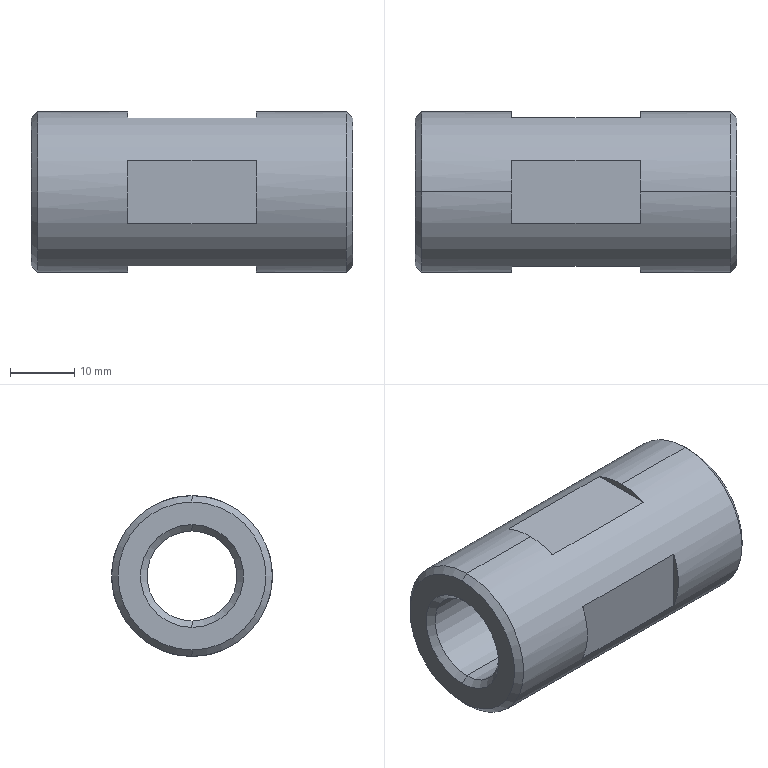Part | SolidWorks | features Chamfer 1, Extrusion 1, HoleWzd 1, ICE 1 | 1 solid | 26 faces | box 50 x 25 x 25 mm | volume 16197 mm3 | plane 14 | cone 8 | cylinder 4 | commonest cylinder face diameters 14 x2 25 x2
STEP:
#1=CARTESIAN_POINT('',(-25.,0.,11.5));
#2=VERTEX_POINT('',#1);
#3=CARTESIAN_POINT('',(-25.,0.,-11.5));
#4=VERTEX_POINT('',#3);
#5=CARTESIAN_POINT('',(-25.,0.,0.));
#6=DIRECTION('',(-1.,0.,0.));
#7=DIRECTION('',(0.,0.,-1.));
#8=AXIS2_PLACEMENT_3D('',#5,#6,#7);
#9=CIRCLE('',#8,11.5);
#10=EDGE_CURVE('',#2,#4,#9,.T.);
#11=ORIENTED_EDGE('',*,*,#10,.F.);
#12=CARTESIAN_POINT('',(-24.,0.,12.5));
#13=VERTEX_POINT('',#12);
#14=CARTESIAN_POINT('',(-24.,0.,12.5));
#15=DIRECTION('',(0.7071,0.,0.7071));
#16=VECTOR('',#15,1000.);
#17=LINE('',#14,#16);
#18=EDGE_CURVE('',#2,#13,#17,.T.);
#19=ORIENTED_EDGE('',*,*,#18,.T.);
#20=CARTESIAN_POINT('',(-24.,0.,-12.5));
#21=VERTEX_POINT('',#20);
#22=CARTESIAN_POINT('',(-24.,0.,0.));
#23=DIRECTION('',(1.,0.,0.));
#24=DIRECTION('',(0.,0.,-1.));
#25=AXIS2_PLACEMENT_3D('',#22,#23,#24);
#26=CIRCLE('',#25,12.5);
#27=EDGE_CURVE('',#21,#13,#26,.T.);
#28=ORIENTED_EDGE('',*,*,#27,.F.);
#29=CARTESIAN_POINT('',(-24.,0.,-12.5));
#30=DIRECTION('',(0.7071,0.,-0.7071));
#31=VECTOR('',#30,1000.);
#32=LINE('',#29,#31);
#33=EDGE_CURVE('',#4,#21,#32,.T.);
#34=ORIENTED_EDGE('',*,*,#33,.F.);
#35=EDGE_LOOP('',(#11,#19,#28,#34));
#36=FACE_OUTER_BOUND('',#35,.T.);
#37=CARTESIAN_POINT('',(-24.,0.,0.));
#38=DIRECTION('',(1.,0.,0.));
#39=DIRECTION('',(0.,0.,-1.));
#40=AXIS2_PLACEMENT_3D('',#37,#38,#39);
#41=CONICAL_SURFACE('',#40,12.5,0.7854);
#42=ADVANCED_FACE('',(#36),#41,.T.);
#43=CARTESIAN_POINT('',(25.,0.,-11.5));
#44=VERTEX_POINT('',#43);
#45=CARTESIAN_POINT('',(25.,0.,11.5));
#46=VERTEX_POINT('',#45);
#47=CARTESIAN_POINT('',(25.,0.,0.));
#48=DIRECTION('',(1.,0.,0.));
#49=DIRECTION('',(0.,0.,-1.));
#50=AXIS2_PLACEMENT_3D('',#47,#48,#49);
#51=CIRCLE('',#50,11.5);
#52=EDGE_CURVE('',#44,#46,#51,.T.);
#53=ORIENTED_EDGE('',*,*,#52,.F.);
#54=CARTESIAN_POINT('',(24.,0.,-12.5));
#55=VERTEX_POINT('',#54);
#56=CARTESIAN_POINT('',(25.,0.,-11.5));
#57=DIRECTION('',(-0.7071,0.,-0.7071));
#58=VECTOR('',#57,1000.);
#59=LINE('',#56,#58);
#60=EDGE_CURVE('',#44,#55,#59,.T.);
#61=ORIENTED_EDGE('',*,*,#60,.T.);
#62=CARTESIAN_POINT('',(24.,0.,12.5));
#63=VERTEX_POINT('',#62);
#64=CARTESIAN_POINT('',(24.,0.,0.));
#65=DIRECTION('',(-1.,0.,0.));
#66=DIRECTION('',(0.,0.,-1.));
#67=AXIS2_PLACEMENT_3D('',#64,#65,#66);
#68=CIRCLE('',#67,12.5);
#69=EDGE_CURVE('',#63,#55,#68,.T.);
#70=ORIENTED_EDGE('',*,*,#69,.F.);
#71=CARTESIAN_POINT('',(25.,0.,11.5));
#72=DIRECTION('',(-0.7071,0.,0.7071));
#73=VECTOR('',#72,1000.);
#74=LINE('',#71,#73);
#75=EDGE_CURVE('',#46,#63,#74,.T.);
#76=ORIENTED_EDGE('',*,*,#75,.F.);
#77=EDGE_LOOP('',(#53,#61,#70,#76));
#78=FACE_OUTER_BOUND('',#77,.T.);
#79=CARTESIAN_POINT('',(25.,0.,0.));
#80=DIRECTION('',(-1.,0.,0.));
#81=DIRECTION('',(0.,0.,1.));
#82=AXIS2_PLACEMENT_3D('',#79,#80,#81);
#83=CONICAL_SURFACE('',#82,11.5,0.7854);
#84=ADVANCED_FACE('',(#78),#83,.T.);
#85=CARTESIAN_POINT('',(24.,0.,7.));
#86=VERTEX_POINT('',#85);
#87=CARTESIAN_POINT('',(24.,0.,-7.));
#88=VERTEX_POINT('',#87);
#89=CARTESIAN_POINT('',(24.,0.,0.));
#90=DIRECTION('',(1.,0.,0.));
#91=DIRECTION('',(0.,0.,-1.));
#92=AXIS2_PLACEMENT_3D('',#89,#90,#91);
#93=CIRCLE('',#92,7.);
#94=EDGE_CURVE('',#86,#88,#93,.T.);
#95=ORIENTED_EDGE('',*,*,#94,.F.);
#96=CARTESIAN_POINT('',(25.,0.,8.));
#97=VERTEX_POINT('',#96);
#98=CARTESIAN_POINT('',(24.,0.,7.));
#99=DIRECTION('',(0.7071,0.,0.7071));
#100=VECTOR('',#99,1000.);
#101=LINE('',#98,#100);
#102=EDGE_CURVE('',#86,#97,#101,.T.);
#103=ORIENTED_EDGE('',*,*,#102,.T.);
#104=CARTESIAN_POINT('',(25.,0.,-8.));
#105=VERTEX_POINT('',#104);
#106=CARTESIAN_POINT('',(25.,0.,0.));
#107=DIRECTION('',(-1.,0.,0.));
#108=DIRECTION('',(0.,0.,-1.));
#109=AXIS2_PLACEMENT_3D('',#106,#107,#108);
#110=CIRCLE('',#109,8.);
#111=EDGE_CURVE('',#105,#97,#110,.T.);
#112=ORIENTED_EDGE('',*,*,#111,.F.);
#113=CARTESIAN_POINT('',(24.,0.,-7.));
#114=DIRECTION('',(0.7071,0.,-0.7071));
#115=VECTOR('',#114,1000.);
#116=LINE('',#113,#115);
#117=EDGE_CURVE('',#88,#105,#116,.T.);
#118=ORIENTED_EDGE('',*,*,#117,.F.);
#119=EDGE_LOOP('',(#95,#103,#112,#118));
#120=FACE_OUTER_BOUND('',#119,.T.);
#121=CARTESIAN_POINT('',(24.,0.,0.));
#122=DIRECTION('',(1.,0.,0.));
#123=DIRECTION('',(0.,0.,-1.));
#124=AXIS2_PLACEMENT_3D('',#121,#122,#123);
#125=CONICAL_SURFACE('',#124,7.,0.7854);
#126=ADVANCED_FACE('',(#120),#125,.F.);
#127=CARTESIAN_POINT('',(-24.,0.,-7.));
#128=VERTEX_POINT('',#127);
#129=CARTESIAN_POINT('',(-24.,0.,7.));
#130=VERTEX_POINT('',#129);
#131=CARTESIAN_POINT('',(-24.,0.,0.));
#132=DIRECTION('',(-1.,0.,0.));
#133=DIRECTION('',(0.,0.,-1.));
#134=AXIS2_PLACEMENT_3D('',#131,#132,#133);
#135=CIRCLE('',#134,7.);
#136=EDGE_CURVE('',#128,#130,#135,.T.);
#137=ORIENTED_EDGE('',*,*,#136,.F.);
#138=CARTESIAN_POINT('',(-25.,0.,-8.));
#139=VERTEX_POINT('',#138);
#140=CARTESIAN_POINT('',(-25.,0.,-8.));
#141=DIRECTION('',(-0.7071,0.,-0.7071));
#142=VECTOR('',#141,1000.);
#143=LINE('',#140,#142);
#144=EDGE_CURVE('',#128,#139,#143,.T.);
#145=ORIENTED_EDGE('',*,*,#144,.T.);
#146=CARTESIAN_POINT('',(-25.,0.,8.));
#147=VERTEX_POINT('',#146);
#148=CARTESIAN_POINT('',(-25.,0.,0.));
#149=DIRECTION('',(1.,0.,0.));
#150=DIRECTION('',(0.,0.,-1.));
#151=AXIS2_PLACEMENT_3D('',#148,#149,#150);
#152=CIRCLE('',#151,8.);
#153=EDGE_CURVE('',#147,#139,#152,.T.);
#154=ORIENTED_EDGE('',*,*,#153,.F.);
#155=CARTESIAN_POINT('',(-25.,0.,8.));
#156=DIRECTION('',(-0.7071,0.,0.7071));
#157=VECTOR('',#156,1000.);
#158=LINE('',#155,#157);
#159=EDGE_CURVE('',#130,#147,#158,.T.);
#160=ORIENTED_EDGE('',*,*,#159,.F.);
#161=EDGE_LOOP('',(#137,#145,#154,#160));
#162=FACE_OUTER_BOUND('',#161,.T.);
#163=CARTESIAN_POINT('',(-25.,0.,0.));
#164=DIRECTION('',(-1.,0.,0.));
#165=DIRECTION('',(0.,0.,1.));
#166=AXIS2_PLACEMENT_3D('',#163,#164,#165);
#167=CONICAL_SURFACE('',#166,8.,0.7854);
#168=ADVANCED_FACE('',(#162),#167,.F.);
#169=ORIENTED_EDGE('',*,*,#136,.T.);
#170=CARTESIAN_POINT('',(25.,0.,7.));
#171=DIRECTION('',(1.,0.,0.));
#172=VECTOR('',#171,1000.);
#173=LINE('',#170,#172);
#174=EDGE_CURVE('',#130,#86,#173,.T.);
#175=ORIENTED_EDGE('',*,*,#174,.T.);
#176=ORIENTED_EDGE('',*,*,#94,.T.);
#177=CARTESIAN_POINT('',(25.,0.,-7.));
#178=DIRECTION('',(1.,0.,0.));
#179=VECTOR('',#178,1000.);
#180=LINE('',#177,#179);
#181=EDGE_CURVE('',#128,#88,#180,.T.);
#182=ORIENTED_EDGE('',*,*,#181,.F.);
#183=EDGE_LOOP('',(#169,#175,#176,#182));
#184=FACE_OUTER_BOUND('',#183,.T.);
#185=CARTESIAN_POINT('',(25.,0.,0.));
#186=DIRECTION('',(1.,0.,0.));
#187=DIRECTION('',(0.,0.,-1.));
#188=AXIS2_PLACEMENT_3D('',#185,#186,#187);
#189=CYLINDRICAL_SURFACE('',#188,7.);
#190=ADVANCED_FACE('',(#184),#189,.F.);
#191=CARTESIAN_POINT('',(10.,11.5,-4.899));
#192=VERTEX_POINT('',#191);
#193=CARTESIAN_POINT('',(-10.,11.5,-4.899));
#194=VERTEX_POINT('',#193);
#195=CARTESIAN_POINT('',(25.,11.5,-4.899));
#196=DIRECTION('',(-1.,0.,0.));
#197=VECTOR('',#196,1000.);
#198=LINE('',#195,#197);
#199=EDGE_CURVE('',#192,#194,#198,.T.);
#200=ORIENTED_EDGE('',*,*,#199,.F.);
#201=CARTESIAN_POINT('',(10.,11.5,4.899));
#202=VERTEX_POINT('',#201);
#203=CARTESIAN_POINT('',(10.,0.,0.));
#204=DIRECTION('',(1.,0.,0.));
#205=DIRECTION('',(0.,0.,-1.));
#206=AXIS2_PLACEMENT_3D('',#203,#204,#205);
#207=CIRCLE('',#206,12.5);
#208=EDGE_CURVE('',#192,#202,#207,.T.);
#209=ORIENTED_EDGE('',*,*,#208,.T.);
#210=CARTESIAN_POINT('',(-10.,11.5,4.899));
#211=VERTEX_POINT('',#210);
#212=CARTESIAN_POINT('',(25.,11.5,4.899));
#213=DIRECTION('',(1.,0.,0.));
#214=VECTOR('',#213,1000.);
#215=LINE('',#212,#214);
#216=EDGE_CURVE('',#211,#202,#215,.T.);
#217=ORIENTED_EDGE('',*,*,#216,.F.);
#218=CARTESIAN_POINT('',(-10.,0.,0.));
#219=DIRECTION('',(1.,0.,0.));
#220=DIRECTION('',(0.,0.,-1.));
#221=AXIS2_PLACEMENT_3D('',#218,#219,#220);
#222=CIRCLE('',#221,12.5);
#223=EDGE_CURVE('',#194,#211,#222,.T.);
#224=ORIENTED_EDGE('',*,*,#223,.F.);
#225=EDGE_LOOP('',(#200,#209,#217,#224));
#226=FACE_BOUND('',#225,.T.);
#227=ORIENTED_EDGE('',*,*,#69,.T.);
#228=CARTESIAN_POINT('',(10.,0.,-12.5));
#229=VERTEX_POINT('',#228);
#230=CARTESIAN_POINT('',(25.,0.,-12.5));
#231=DIRECTION('',(-1.,0.,0.));
#232=VECTOR('',#231,1000.);
#233=LINE('',#230,#232);
#234=EDGE_CURVE('',#55,#229,#233,.T.);
#235=ORIENTED_EDGE('',*,*,#234,.T.);
#236=CARTESIAN_POINT('',(10.,4.899,-11.5));
#237=VERTEX_POINT('',#236);
#238=CARTESIAN_POINT('',(10.,0.,0.));
#239=DIRECTION('',(1.,0.,0.));
#240=DIRECTION('',(0.,0.,-1.));
#241=AXIS2_PLACEMENT_3D('',#238,#239,#240);
#242=CIRCLE('',#241,12.5);
#243=EDGE_CURVE('',#229,#237,#242,.T.);
#244=ORIENTED_EDGE('',*,*,#243,.T.);
#245=CARTESIAN_POINT('',(-10.,4.899,-11.5));
#246=VERTEX_POINT('',#245);
#247=CARTESIAN_POINT('',(25.,4.899,-11.5));
#248=DIRECTION('',(1.,0.,0.));
#249=VECTOR('',#248,1000.);
#250=LINE('',#247,#249);
#251=EDGE_CURVE('',#246,#237,#250,.T.);
#252=ORIENTED_EDGE('',*,*,#251,.F.);
#253=CARTESIAN_POINT('',(-10.,0.,-12.5));
#254=VERTEX_POINT('',#253);
#255=CARTESIAN_POINT('',(-10.,0.,0.));
#256=DIRECTION('',(1.,0.,0.));
#257=DIRECTION('',(0.,0.,-1.));
#258=AXIS2_PLACEMENT_3D('',#255,#256,#257);
#259=CIRCLE('',#258,12.5);
#260=EDGE_CURVE('',#254,#246,#259,.T.);
#261=ORIENTED_EDGE('',*,*,#260,.F.);
#262=CARTESIAN_POINT('',(25.,0.,-12.5));
#263=DIRECTION('',(-1.,0.,0.));
#264=VECTOR('',#263,1000.);
#265=LINE('',#262,#264);
#266=EDGE_CURVE('',#254,#21,#265,.T.);
#267=ORIENTED_EDGE('',*,*,#266,.T.);
#268=ORIENTED_EDGE('',*,*,#27,.T.);
#269=CARTESIAN_POINT('',(-10.,0.,12.5));
#270=VERTEX_POINT('',#269);
#271=CARTESIAN_POINT('',(25.,0.,12.5));
#272=DIRECTION('',(-1.,0.,0.));
#273=VECTOR('',#272,1000.);
#274=LINE('',#271,#273);
#275=EDGE_CURVE('',#270,#13,#274,.T.);
#276=ORIENTED_EDGE('',*,*,#275,.F.);
#277=CARTESIAN_POINT('',(-10.,4.899,11.5));
#278=VERTEX_POINT('',#277);
#279=CARTESIAN_POINT('',(-10.,0.,0.));
#280=DIRECTION('',(1.,0.,0.));
#281=DIRECTION('',(0.,0.,-1.));
#282=AXIS2_PLACEMENT_3D('',#279,#280,#281);
#283=CIRCLE('',#282,12.5);
#284=EDGE_CURVE('',#278,#270,#283,.T.);
#285=ORIENTED_EDGE('',*,*,#284,.F.);
#286=CARTESIAN_POINT('',(10.,4.899,11.5));
#287=VERTEX_POINT('',#286);
#288=CARTESIAN_POINT('',(25.,4.899,11.5));
#289=DIRECTION('',(-1.,0.,0.));
#290=VECTOR('',#289,1000.);
#291=LINE('',#288,#290);
#292=EDGE_CURVE('',#287,#278,#291,.T.);
#293=ORIENTED_EDGE('',*,*,#292,.F.);
#294=CARTESIAN_POINT('',(10.,0.,12.5));
#295=VERTEX_POINT('',#294);
#296=CARTESIAN_POINT('',(10.,0.,0.));
#297=DIRECTION('',(1.,0.,0.));
#298=DIRECTION('',(0.,0.,-1.));
#299=AXIS2_PLACEMENT_3D('',#296,#297,#298);
#300=CIRCLE('',#299,12.5);
#301=EDGE_CURVE('',#287,#295,#300,.T.);
#302=ORIENTED_EDGE('',*,*,#301,.T.);
#303=CARTESIAN_POINT('',(25.,0.,12.5));
#304=DIRECTION('',(-1.,0.,0.));
#305=VECTOR('',#304,1000.);
#306=LINE('',#303,#305);
#307=EDGE_CURVE('',#63,#295,#306,.T.);
#308=ORIENTED_EDGE('',*,*,#307,.F.);
#309=EDGE_LOOP('',(#227,#235,#244,#252,#261,#267,#268,#276,#285,#293,#302,#308));
#310=FACE_OUTER_BOUND('',#309,.T.);
#311=CARTESIAN_POINT('',(25.,0.,0.));
#312=DIRECTION('',(-1.,0.,0.));
#313=DIRECTION('',(0.,0.,1.));
#314=AXIS2_PLACEMENT_3D('',#311,#312,#313);
#315=CYLINDRICAL_SURFACE('',#314,12.5);
#316=ADVANCED_FACE('',(#226,#310),#315,.T.);
#317=ORIENTED_EDGE('',*,*,#234,.F.);
#318=CARTESIAN_POINT('',(24.,0.,0.));
#319=DIRECTION('',(-1.,0.,0.));
#320=DIRECTION('',(0.,0.,-1.));
#321=AXIS2_PLACEMENT_3D('',#318,#319,#320);
#322=CIRCLE('',#321,12.5);
#323=EDGE_CURVE('',#55,#63,#322,.T.);
#324=ORIENTED_EDGE('',*,*,#323,.T.);
#325=ORIENTED_EDGE('',*,*,#307,.T.);
#326=CARTESIAN_POINT('',(10.,-4.899,11.5));
#327=VERTEX_POINT('',#326);
#328=CARTESIAN_POINT('',(10.,0.,0.));
#329=DIRECTION('',(1.,0.,0.));
#330=DIRECTION('',(0.,0.,-1.));
#331=AXIS2_PLACEMENT_3D('',#328,#329,#330);
#332=CIRCLE('',#331,12.5);
#333=EDGE_CURVE('',#295,#327,#332,.T.);
#334=ORIENTED_EDGE('',*,*,#333,.T.);
#335=CARTESIAN_POINT('',(-10.,-4.899,11.5));
#336=VERTEX_POINT('',#335);
#337=CARTESIAN_POINT('',(25.,-4.899,11.5));
#338=DIRECTION('',(1.,0.,0.));
#339=VECTOR('',#338,1000.);
#340=LINE('',#337,#339);
#341=EDGE_CURVE('',#336,#327,#340,.T.);
#342=ORIENTED_EDGE('',*,*,#341,.F.);
#343=CARTESIAN_POINT('',(-10.,0.,0.));
#344=DIRECTION('',(1.,0.,0.));
#345=DIRECTION('',(0.,0.,-1.));
#346=AXIS2_PLACEMENT_3D('',#343,#344,#345);
#347=CIRCLE('',#346,12.5);
#348=EDGE_CURVE('',#270,#336,#347,.T.);
#349=ORIENTED_EDGE('',*,*,#348,.F.);
#350=ORIENTED_EDGE('',*,*,#275,.T.);
#351=CARTESIAN_POINT('',(-24.,0.,0.));
#352=DIRECTION('',(1.,0.,0.));
#353=DIRECTION('',(0.,0.,-1.));
#354=AXIS2_PLACEMENT_3D('',#351,#352,#353);
#355=CIRCLE('',#354,12.5);
#356=EDGE_CURVE('',#13,#21,#355,.T.);
#357=ORIENTED_EDGE('',*,*,#356,.T.);
#358=ORIENTED_EDGE('',*,*,#266,.F.);
#359=CARTESIAN_POINT('',(-10.,-4.899,-11.5));
#360=VERTEX_POINT('',#359);
#361=CARTESIAN_POINT('',(-10.,0.,0.));
#362=DIRECTION('',(1.,0.,0.));
#363=DIRECTION('',(0.,0.,-1.));
#364=AXIS2_PLACEMENT_3D('',#361,#362,#363);
#365=CIRCLE('',#364,12.5);
#366=EDGE_CURVE('',#360,#254,#365,.T.);
#367=ORIENTED_EDGE('',*,*,#366,.F.);
#368=CARTESIAN_POINT('',(10.,-4.899,-11.5));
#369=VERTEX_POINT('',#368);
#370=CARTESIAN_POINT('',(25.,-4.899,-11.5));
#371=DIRECTION('',(-1.,0.,0.));
#372=VECTOR('',#371,1000.);
#373=LINE('',#370,#372);
#374=EDGE_CURVE('',#369,#360,#373,.T.);
#375=ORIENTED_EDGE('',*,*,#374,.F.);
#376=CARTESIAN_POINT('',(10.,0.,0.));
#377=DIRECTION('',(1.,0.,0.));
#378=DIRECTION('',(0.,0.,-1.));
#379=AXIS2_PLACEMENT_3D('',#376,#377,#378);
#380=CIRCLE('',#379,12.5);
#381=EDGE_CURVE('',#369,#229,#380,.T.);
#382=ORIENTED_EDGE('',*,*,#381,.T.);
#383=EDGE_LOOP('',(#317,#324,#325,#334,#342,#349,#350,#357,#358,#367,#375,#382));
#384=FACE_OUTER_BOUND('',#383,.T.);
#385=CARTESIAN_POINT('',(10.,-11.5,4.899));
#386=VERTEX_POINT('',#385);
#387=CARTESIAN_POINT('',(-10.,-11.5,4.899));
#388=VERTEX_POINT('',#387);
#389=CARTESIAN_POINT('',(25.,-11.5,4.899));
#390=DIRECTION('',(-1.,0.,0.));
#391=VECTOR('',#390,1000.);
#392=LINE('',#389,#391);
#393=EDGE_CURVE('',#386,#388,#392,.T.);
#394=ORIENTED_EDGE('',*,*,#393,.F.);
#395=CARTESIAN_POINT('',(10.,-11.5,-4.899));
#396=VERTEX_POINT('',#395);
#397=CARTESIAN_POINT('',(10.,0.,0.));
#398=DIRECTION('',(1.,0.,0.));
#399=DIRECTION('',(0.,0.,-1.));
#400=AXIS2_PLACEMENT_3D('',#397,#398,#399);
#401=CIRCLE('',#400,12.5);
#402=EDGE_CURVE('',#386,#396,#401,.T.);
#403=ORIENTED_EDGE('',*,*,#402,.T.);
#404=CARTESIAN_POINT('',(-10.,-11.5,-4.899));
#405=VERTEX_POINT('',#404);
#406=CARTESIAN_POINT('',(25.,-11.5,-4.899));
#407=DIRECTION('',(1.,0.,0.));
#408=VECTOR('',#407,1000.);
#409=LINE('',#406,#408);
#410=EDGE_CURVE('',#405,#396,#409,.T.);
#411=ORIENTED_EDGE('',*,*,#410,.F.);
#412=CARTESIAN_POINT('',(-10.,0.,0.));
#413=DIRECTION('',(1.,0.,0.));
#414=DIRECTION('',(0.,0.,-1.));
#415=AXIS2_PLACEMENT_3D('',#412,#413,#414);
#416=CIRCLE('',#415,12.5);
#417=EDGE_CURVE('',#388,#405,#416,.T.);
#418=ORIENTED_EDGE('',*,*,#417,.F.);
#419=EDGE_LOOP('',(#394,#403,#411,#418));
#420=FACE_BOUND('',#419,.T.);
#421=CARTESIAN_POINT('',(25.,0.,0.));
#422=DIRECTION('',(-1.,0.,0.));
#423=DIRECTION('',(0.,0.,1.));
#424=AXIS2_PLACEMENT_3D('',#421,#422,#423);
#425=CYLINDRICAL_SURFACE('',#424,12.5);
#426=ADVANCED_FACE('',(#384,#420),#425,.T.);
#427=ORIENTED_EDGE('',*,*,#111,.T.);
#428=CARTESIAN_POINT('',(25.,0.,0.));
#429=DIRECTION('',(-1.,0.,0.));
#430=DIRECTION('',(0.,0.,-1.));
#431=AXIS2_PLACEMENT_3D('',#428,#429,#430);
#432=CIRCLE('',#431,8.);
#433=EDGE_CURVE('',#97,#105,#432,.T.);
#434=ORIENTED_EDGE('',*,*,#433,.T.);
#435=EDGE_LOOP('',(#427,#434));
#436=FACE_BOUND('',#435,.T.);
#437=CARTESIAN_POINT('',(25.,0.,0.));
#438=DIRECTION('',(1.,0.,0.));
#439=DIRECTION('',(0.,0.,-1.));
#440=AXIS2_PLACEMENT_3D('',#437,#438,#439);
#441=CIRCLE('',#440,11.5);
#442=EDGE_CURVE('',#46,#44,#441,.T.);
#443=ORIENTED_EDGE('',*,*,#442,.T.);
#444=ORIENTED_EDGE('',*,*,#52,.T.);
#445=EDGE_LOOP('',(#443,#444));
#446=FACE_OUTER_BOUND('',#445,.T.);
#447=CARTESIAN_POINT('',(25.,0.,0.));
#448=DIRECTION('',(1.,0.,0.));
#449=DIRECTION('',(0.,0.,-1.));
#450=AXIS2_PLACEMENT_3D('',#447,#448,#449);
#451=PLANE('',#450);
#452=ADVANCED_FACE('',(#436,#446),#451,.T.);
#453=ORIENTED_EDGE('',*,*,#153,.T.);
#454=CARTESIAN_POINT('',(-25.,0.,0.));
#455=DIRECTION('',(1.,0.,0.));
#456=DIRECTION('',(0.,0.,-1.));
#457=AXIS2_PLACEMENT_3D('',#454,#455,#456);
#458=CIRCLE('',#457,8.);
#459=EDGE_CURVE('',#139,#147,#458,.T.);
#460=ORIENTED_EDGE('',*,*,#459,.T.);
#461=EDGE_LOOP('',(#453,#460));
#462=FACE_BOUND('',#461,.T.);
#463=CARTESIAN_POINT('',(-25.,0.,0.));
#464=DIRECTION('',(-1.,0.,0.));
#465=DIRECTION('',(0.,0.,-1.));
#466=AXIS2_PLACEMENT_3D('',#463,#464,#465);
#467=CIRCLE('',#466,11.5);
#468=EDGE_CURVE('',#4,#2,#467,.T.);
#469=ORIENTED_EDGE('',*,*,#468,.T.);
#470=ORIENTED_EDGE('',*,*,#10,.T.);
#471=EDGE_LOOP('',(#469,#470));
#472=FACE_OUTER_BOUND('',#471,.T.);
#473=CARTESIAN_POINT('',(-25.,0.,0.));
#474=DIRECTION('',(1.,0.,0.));
#475=DIRECTION('',(0.,0.,-1.));
#476=AXIS2_PLACEMENT_3D('',#473,#474,#475);
#477=PLANE('',#476);
#478=ADVANCED_FACE('',(#462,#472),#477,.F.);
#479=ORIENTED_EDGE('',*,*,#174,.F.);
#480=CARTESIAN_POINT('',(-24.,0.,0.));
#481=DIRECTION('',(-1.,0.,0.));
#482=DIRECTION('',(0.,0.,-1.));
#483=AXIS2_PLACEMENT_3D('',#480,#481,#482);
#484=CIRCLE('',#483,7.);
#485=EDGE_CURVE('',#130,#128,#484,.T.);
#486=ORIENTED_EDGE('',*,*,#485,.T.);
#487=ORIENTED_EDGE('',*,*,#181,.T.);
#488=CARTESIAN_POINT('',(24.,0.,0.));
#489=DIRECTION('',(1.,0.,0.));
#490=DIRECTION('',(0.,0.,-1.));
#491=AXIS2_PLACEMENT_3D('',#488,#489,#490);
#492=CIRCLE('',#491,7.);
#493=EDGE_CURVE('',#88,#86,#492,.T.);
#494=ORIENTED_EDGE('',*,*,#493,.T.);
#495=EDGE_LOOP('',(#479,#486,#487,#494));
#496=FACE_OUTER_BOUND('',#495,.T.);
#497=CARTESIAN_POINT('',(25.,0.,0.));
#498=DIRECTION('',(1.,0.,0.));
#499=DIRECTION('',(0.,0.,-1.));
#500=AXIS2_PLACEMENT_3D('',#497,#498,#499);
#501=CYLINDRICAL_SURFACE('',#500,7.);
#502=ADVANCED_FACE('',(#496),#501,.F.);
#503=ORIENTED_EDGE('',*,*,#199,.T.);
#504=CARTESIAN_POINT('',(-10.,11.5,11.5));
#505=DIRECTION('',(0.,0.,1.));
#506=VECTOR('',#505,1000.);
#507=LINE('',#504,#506);
#508=EDGE_CURVE('',#194,#211,#507,.T.);
#509=ORIENTED_EDGE('',*,*,#508,.T.);
#510=ORIENTED_EDGE('',*,*,#216,.T.);
#511=CARTESIAN_POINT('',(10.,11.5,11.5));
#512=DIRECTION('',(0.,0.,1.));
#513=VECTOR('',#512,1000.);
#514=LINE('',#511,#513);
#515=EDGE_CURVE('',#192,#202,#514,.T.);
#516=ORIENTED_EDGE('',*,*,#515,.F.);
#517=EDGE_LOOP('',(#503,#509,#510,#516));
#518=FACE_OUTER_BOUND('',#517,.T.);
#519=CARTESIAN_POINT('',(-10.,11.5,11.5));
#520=DIRECTION('',(0.,1.,0.));
#521=DIRECTION('',(0.,0.,1.));
#522=AXIS2_PLACEMENT_3D('',#519,#520,#521);
#523=PLANE('',#522);
#524=ADVANCED_FACE('',(#518),#523,.T.);
#525=ORIENTED_EDGE('',*,*,#515,.T.);
#526=ORIENTED_EDGE('',*,*,#208,.F.);
#527=EDGE_LOOP('',(#525,#526));
#528=FACE_OUTER_BOUND('',#527,.T.);
#529=CARTESIAN_POINT('',(10.,0.,0.));
#530=DIRECTION('',(1.,0.,0.));
#531=DIRECTION('',(0.,0.,-1.));
#532=AXIS2_PLACEMENT_3D('',#529,#530,#531);
#533=PLANE('',#532);
#534=ADVANCED_FACE('',(#528),#533,.F.);
#535=ORIENTED_EDGE('',*,*,#223,.T.);
#536=ORIENTED_EDGE('',*,*,#508,.F.);
#537=EDGE_LOOP('',(#535,#536));
#538=FACE_OUTER_BOUND('',#537,.T.);
#539=CARTESIAN_POINT('',(-10.,0.,0.));
#540=DIRECTION('',(1.,0.,0.));
#541=DIRECTION('',(0.,0.,-1.));
#542=AXIS2_PLACEMENT_3D('',#539,#540,#541);
#543=PLANE('',#542);
#544=ADVANCED_FACE('',(#538),#543,.T.);
#545=ORIENTED_EDGE('',*,*,#292,.T.);
#546=CARTESIAN_POINT('',(-10.,11.5,11.5));
#547=DIRECTION('',(0.,-1.,0.));
#548=VECTOR('',#547,1000.);
#549=LINE('',#546,#548);
#550=EDGE_CURVE('',#278,#336,#549,.T.);
#551=ORIENTED_EDGE('',*,*,#550,.T.);
#552=ORIENTED_EDGE('',*,*,#341,.T.);
#553=CARTESIAN_POINT('',(10.,11.5,11.5));
#554=DIRECTION('',(0.,-1.,0.));
#555=VECTOR('',#554,1000.);
#556=LINE('',#553,#555);
#557=EDGE_CURVE('',#287,#327,#556,.T.);
#558=ORIENTED_EDGE('',*,*,#557,.F.);
#559=EDGE_LOOP('',(#545,#551,#552,#558));
#560=FACE_OUTER_BOUND('',#559,.T.);
#561=CARTESIAN_POINT('',(-10.,11.5,11.5));
#562=DIRECTION('',(0.,0.,1.));
#563=DIRECTION('',(0.,-1.,0.));
#564=AXIS2_PLACEMENT_3D('',#561,#562,#563);
#565=PLANE('',#564);
#566=ADVANCED_FACE('',(#560),#565,.T.);
#567=ORIENTED_EDGE('',*,*,#557,.T.);
#568=ORIENTED_EDGE('',*,*,#333,.F.);
#569=ORIENTED_EDGE('',*,*,#301,.F.);
#570=EDGE_LOOP('',(#567,#568,#569));
#571=FACE_OUTER_BOUND('',#570,.T.);
#572=CARTESIAN_POINT('',(10.,0.,0.));
#573=DIRECTION('',(1.,0.,0.));
#574=DIRECTION('',(0.,0.,-1.));
#575=AXIS2_PLACEMENT_3D('',#572,#573,#574);
#576=PLANE('',#575);
#577=ADVANCED_FACE('',(#571),#576,.F.);
#578=ORIENTED_EDGE('',*,*,#284,.T.);
#579=ORIENTED_EDGE('',*,*,#348,.T.);
#580=ORIENTED_EDGE('',*,*,#550,.F.);
#581=EDGE_LOOP('',(#578,#579,#580));
#582=FACE_OUTER_BOUND('',#581,.T.);
#583=CARTESIAN_POINT('',(-10.,0.,0.));
#584=DIRECTION('',(1.,0.,0.));
#585=DIRECTION('',(0.,0.,-1.));
#586=AXIS2_PLACEMENT_3D('',#583,#584,#585);
#587=PLANE('',#586);
#588=ADVANCED_FACE('',(#582),#587,.T.);
#589=ORIENTED_EDGE('',*,*,#393,.T.);
#590=CARTESIAN_POINT('',(-10.,-11.5,11.5));
#591=DIRECTION('',(0.,0.,-1.));
#592=VECTOR('',#591,1000.);
#593=LINE('',#590,#592);
#594=EDGE_CURVE('',#388,#405,#593,.T.);
#595=ORIENTED_EDGE('',*,*,#594,.T.);
#596=ORIENTED_EDGE('',*,*,#410,.T.);
#597=CARTESIAN_POINT('',(10.,-11.5,11.5));
#598=DIRECTION('',(0.,0.,-1.));
#599=VECTOR('',#598,1000.);
#600=LINE('',#597,#599);
#601=EDGE_CURVE('',#386,#396,#600,.T.);
#602=ORIENTED_EDGE('',*,*,#601,.F.);
#603=EDGE_LOOP('',(#589,#595,#596,#602));
#604=FACE_OUTER_BOUND('',#603,.T.);
#605=CARTESIAN_POINT('',(-10.,-11.5,11.5));
#606=DIRECTION('',(0.,-1.,0.));
#607=DIRECTION('',(0.,0.,-1.));
#608=AXIS2_PLACEMENT_3D('',#605,#606,#607);
#609=PLANE('',#608);
#610=ADVANCED_FACE('',(#604),#609,.T.);
#611=ORIENTED_EDGE('',*,*,#601,.T.);
#612=ORIENTED_EDGE('',*,*,#402,.F.);
#613=EDGE_LOOP('',(#611,#612));
#614=FACE_OUTER_BOUND('',#613,.T.);
#615=CARTESIAN_POINT('',(10.,0.,0.));
#616=DIRECTION('',(1.,0.,0.));
#617=DIRECTION('',(0.,0.,-1.));
#618=AXIS2_PLACEMENT_3D('',#615,#616,#617);
#619=PLANE('',#618);
#620=ADVANCED_FACE('',(#614),#619,.F.);
#621=ORIENTED_EDGE('',*,*,#417,.T.);
#622=ORIENTED_EDGE('',*,*,#594,.F.);
#623=EDGE_LOOP('',(#621,#622));
#624=FACE_OUTER_BOUND('',#623,.T.);
#625=CARTESIAN_POINT('',(-10.,0.,0.));
#626=DIRECTION('',(1.,0.,0.));
#627=DIRECTION('',(0.,0.,-1.));
#628=AXIS2_PLACEMENT_3D('',#625,#626,#627);
#629=PLANE('',#628);
#630=ADVANCED_FACE('',(#624),#629,.T.);
#631=ORIENTED_EDGE('',*,*,#366,.T.);
#632=ORIENTED_EDGE('',*,*,#260,.T.);
#633=CARTESIAN_POINT('',(-10.,11.5,-11.5));
#634=DIRECTION('',(0.,1.,0.));
#635=VECTOR('',#634,1000.);
#636=LINE('',#633,#635);
#637=EDGE_CURVE('',#360,#246,#636,.T.);
#638=ORIENTED_EDGE('',*,*,#637,.F.);
#639=EDGE_LOOP('',(#631,#632,#638));
#640=FACE_OUTER_BOUND('',#639,.T.);
#641=CARTESIAN_POINT('',(-10.,0.,0.));
#642=DIRECTION('',(1.,0.,0.));
#643=DIRECTION('',(0.,0.,-1.));
#644=AXIS2_PLACEMENT_3D('',#641,#642,#643);
#645=PLANE('',#644);
#646=ADVANCED_FACE('',(#640),#645,.T.);
#647=CARTESIAN_POINT('',(10.,11.5,-11.5));
#648=DIRECTION('',(0.,1.,0.));
#649=VECTOR('',#648,1000.);
#650=LINE('',#647,#649);
#651=EDGE_CURVE('',#369,#237,#650,.T.);
#652=ORIENTED_EDGE('',*,*,#651,.T.);
#653=ORIENTED_EDGE('',*,*,#243,.F.);
#654=ORIENTED_EDGE('',*,*,#381,.F.);
#655=EDGE_LOOP('',(#652,#653,#654));
#656=FACE_OUTER_BOUND('',#655,.T.);
#657=CARTESIAN_POINT('',(10.,0.,0.));
#658=DIRECTION('',(1.,0.,0.));
#659=DIRECTION('',(0.,0.,-1.));
#660=AXIS2_PLACEMENT_3D('',#657,#658,#659);
#661=PLANE('',#660);
#662=ADVANCED_FACE('',(#656),#661,.F.);
#663=ORIENTED_EDGE('',*,*,#374,.T.);
#664=ORIENTED_EDGE('',*,*,#637,.T.);
#665=ORIENTED_EDGE('',*,*,#251,.T.);
#666=ORIENTED_EDGE('',*,*,#651,.F.);
#667=EDGE_LOOP('',(#663,#664,#665,#666));
#668=FACE_OUTER_BOUND('',#667,.T.);
#669=CARTESIAN_POINT('',(-10.,11.5,-11.5));
#670=DIRECTION('',(0.,0.,-1.));
#671=DIRECTION('',(0.,1.,0.));
#672=AXIS2_PLACEMENT_3D('',#669,#670,#671);
#673=PLANE('',#672);
#674=ADVANCED_FACE('',(#668),#673,.T.);
#675=ORIENTED_EDGE('',*,*,#144,.F.);
#676=ORIENTED_EDGE('',*,*,#485,.F.);
#677=ORIENTED_EDGE('',*,*,#159,.T.);
#678=ORIENTED_EDGE('',*,*,#459,.F.);
#679=EDGE_LOOP('',(#675,#676,#677,#678));
#680=FACE_OUTER_BOUND('',#679,.T.);
#681=CARTESIAN_POINT('',(-25.,0.,0.));
#682=DIRECTION('',(-1.,0.,0.));
#683=DIRECTION('',(0.,0.,1.));
#684=AXIS2_PLACEMENT_3D('',#681,#682,#683);
#685=CONICAL_SURFACE('',#684,8.,0.7854);
#686=ADVANCED_FACE('',(#680),#685,.F.);
#687=ORIENTED_EDGE('',*,*,#102,.F.);
#688=ORIENTED_EDGE('',*,*,#493,.F.);
#689=ORIENTED_EDGE('',*,*,#117,.T.);
#690=ORIENTED_EDGE('',*,*,#433,.F.);
#691=EDGE_LOOP('',(#687,#688,#689,#690));
#692=FACE_OUTER_BOUND('',#691,.T.);
#693=CARTESIAN_POINT('',(24.,0.,0.));
#694=DIRECTION('',(1.,0.,0.));
#695=DIRECTION('',(0.,0.,-1.));
#696=AXIS2_PLACEMENT_3D('',#693,#694,#695);
#697=CONICAL_SURFACE('',#696,7.,0.7854);
#698=ADVANCED_FACE('',(#692),#697,.F.);
#699=ORIENTED_EDGE('',*,*,#60,.F.);
#700=ORIENTED_EDGE('',*,*,#442,.F.);
#701=ORIENTED_EDGE('',*,*,#75,.T.);
#702=ORIENTED_EDGE('',*,*,#323,.F.);
#703=EDGE_LOOP('',(#699,#700,#701,#702));
#704=FACE_OUTER_BOUND('',#703,.T.);
#705=CARTESIAN_POINT('',(25.,0.,0.));
#706=DIRECTION('',(-1.,0.,0.));
#707=DIRECTION('',(0.,0.,1.));
#708=AXIS2_PLACEMENT_3D('',#705,#706,#707);
#709=CONICAL_SURFACE('',#708,11.5,0.7854);
#710=ADVANCED_FACE('',(#704),#709,.T.);
#711=ORIENTED_EDGE('',*,*,#18,.F.);
#712=ORIENTED_EDGE('',*,*,#468,.F.);
#713=ORIENTED_EDGE('',*,*,#33,.T.);
#714=ORIENTED_EDGE('',*,*,#356,.F.);
#715=EDGE_LOOP('',(#711,#712,#713,#714));
#716=FACE_OUTER_BOUND('',#715,.T.);
#717=CARTESIAN_POINT('',(-24.,0.,0.));
#718=DIRECTION('',(1.,0.,0.));
#719=DIRECTION('',(0.,0.,-1.));
#720=AXIS2_PLACEMENT_3D('',#717,#718,#719);
#721=CONICAL_SURFACE('',#720,12.5,0.7854);
#722=ADVANCED_FACE('',(#716),#721,.T.);
#723=CLOSED_SHELL('',(#42,#84,#126,#168,#190,#316,#426,#452,#478,#502,#524,#534,#544,#566,#577,#588,#610,#620,#630,#646,#662,#674,#686,#698,#710,#722));
#724=MANIFOLD_SOLID_BREP('',#723);
#725=CARTESIAN_POINT('',(0.,0.,0.));
#726=DIRECTION('',(0.,0.,1.));
#727=DIRECTION('',(1.,0.,0.));
#728=AXIS2_PLACEMENT_3D('',#725,#726,#727);
#729=(LENGTH_UNIT()NAMED_UNIT(*)SI_UNIT(.MILLI.,.METRE.));
#730=UNCERTAINTY_MEASURE_WITH_UNIT(LENGTH_MEASURE(0.00001),#729,'','');
#731=(NAMED_UNIT(*)PLANE_ANGLE_UNIT()SI_UNIT($,.RADIAN.));
#732=(NAMED_UNIT(*)SI_UNIT($,.STERADIAN.)SOLID_ANGLE_UNIT());
#733=(GEOMETRIC_REPRESENTATION_CONTEXT(3)GLOBAL_UNCERTAINTY_ASSIGNED_CONTEXT((#730))GLOBAL_UNIT_ASSIGNED_CONTEXT((#729,#731,#732))REPRESENTATION_CONTEXT('',''));
#734=ADVANCED_BREP_SHAPE_REPRESENTATION('',(#724,#728),#733);